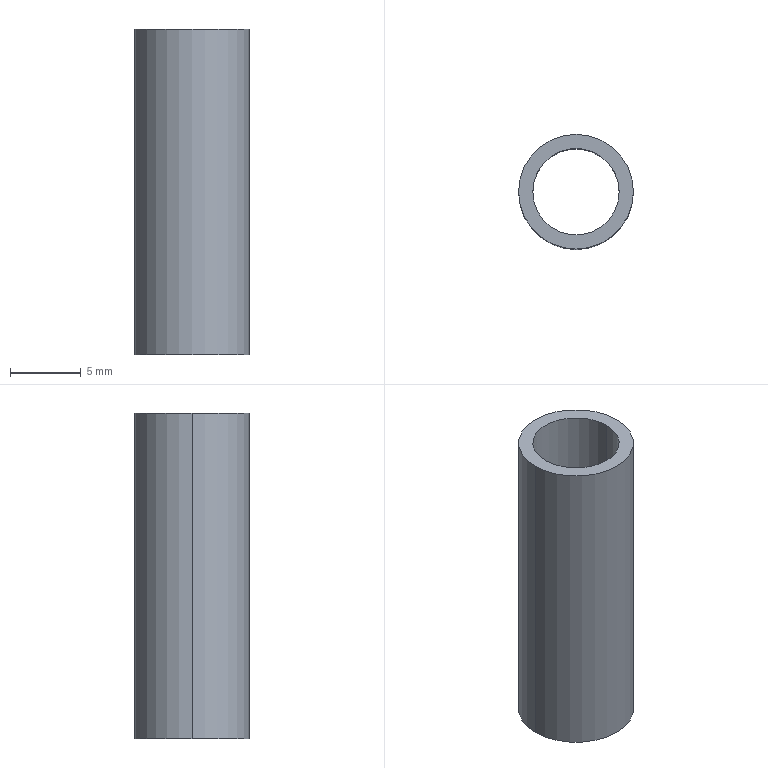Part | NX | features BREP 1 | 1 solid | 6 faces | box 8.1 x 8.1 x 23 mm | volume 513.022 mm3 | cylinder 4 | plane 2 | commonest cylinder face diameters 6.1 x2 8.1 x2
STEP:
#1=CARTESIAN_POINT('',(144.219,-518.178,23.));
#2=VERTEX_POINT('',#1);
#3=CARTESIAN_POINT('',(150.319,-518.178,23.));
#4=VERTEX_POINT('',#3);
#5=CARTESIAN_POINT('',(147.269,-518.178,23.));
#6=DIRECTION('',(0.,0.,1.));
#7=DIRECTION('',(0.,-1.,0.));
#8=AXIS2_PLACEMENT_3D('',#5,#6,#7);
#9=CIRCLE('',#8,3.05);
#10=EDGE_CURVE('',#2,#4,#9,.T.);
#11=ORIENTED_EDGE('',*,*,#10,.T.);
#12=CARTESIAN_POINT('',(150.319,-518.178,0.));
#13=VERTEX_POINT('',#12);
#14=CARTESIAN_POINT('',(150.319,-518.178,34.455));
#15=DIRECTION('',(0.,0.,-1.));
#16=VECTOR('',#15,1000.);
#17=LINE('',#14,#16);
#18=EDGE_CURVE('',#13,#4,#17,.F.);
#19=ORIENTED_EDGE('',*,*,#18,.F.);
#20=CARTESIAN_POINT('',(144.219,-518.178,0.));
#21=VERTEX_POINT('',#20);
#22=CARTESIAN_POINT('',(147.269,-518.178,0.));
#23=DIRECTION('',(0.,0.,1.));
#24=DIRECTION('',(1.,0.,0.));
#25=AXIS2_PLACEMENT_3D('',#22,#23,#24);
#26=CIRCLE('',#25,3.05);
#27=EDGE_CURVE('',#21,#13,#26,.T.);
#28=ORIENTED_EDGE('',*,*,#27,.F.);
#29=CARTESIAN_POINT('',(144.219,-518.178,34.455));
#30=DIRECTION('',(0.,0.,-1.));
#31=VECTOR('',#30,1000.);
#32=LINE('',#29,#31);
#33=EDGE_CURVE('',#21,#2,#32,.F.);
#34=ORIENTED_EDGE('',*,*,#33,.T.);
#35=EDGE_LOOP('',(#11,#19,#28,#34));
#36=FACE_BOUND('',#35,.T.);
#37=CARTESIAN_POINT('',(147.269,-518.178,34.455));
#38=DIRECTION('',(0.,0.,-1.));
#39=DIRECTION('',(1.,0.,0.));
#40=AXIS2_PLACEMENT_3D('',#37,#38,#39);
#41=CYLINDRICAL_SURFACE('',#40,3.05);
#42=ADVANCED_FACE('',(#36),#41,.F.);
#43=CARTESIAN_POINT('',(151.319,-518.178,23.));
#44=VERTEX_POINT('',#43);
#45=CARTESIAN_POINT('',(143.219,-518.178,23.));
#46=VERTEX_POINT('',#45);
#47=CARTESIAN_POINT('',(147.269,-518.178,23.));
#48=DIRECTION('',(0.,0.,1.));
#49=DIRECTION('',(0.,-1.,0.));
#50=AXIS2_PLACEMENT_3D('',#47,#48,#49);
#51=CIRCLE('',#50,4.05);
#52=EDGE_CURVE('',#44,#46,#51,.T.);
#53=ORIENTED_EDGE('',*,*,#52,.F.);
#54=CARTESIAN_POINT('',(151.319,-518.178,0.));
#55=VERTEX_POINT('',#54);
#56=CARTESIAN_POINT('',(151.319,-518.178,34.455));
#57=DIRECTION('',(0.,0.,-1.));
#58=VECTOR('',#57,1000.);
#59=LINE('',#56,#58);
#60=EDGE_CURVE('',#55,#44,#59,.F.);
#61=ORIENTED_EDGE('',*,*,#60,.F.);
#62=CARTESIAN_POINT('',(143.219,-518.178,0.));
#63=VERTEX_POINT('',#62);
#64=CARTESIAN_POINT('',(147.269,-518.178,0.));
#65=DIRECTION('',(0.,0.,1.));
#66=DIRECTION('',(1.,0.,0.));
#67=AXIS2_PLACEMENT_3D('',#64,#65,#66);
#68=CIRCLE('',#67,4.05);
#69=EDGE_CURVE('',#55,#63,#68,.T.);
#70=ORIENTED_EDGE('',*,*,#69,.T.);
#71=CARTESIAN_POINT('',(143.219,-518.178,34.455));
#72=DIRECTION('',(0.,0.,-1.));
#73=VECTOR('',#72,1000.);
#74=LINE('',#71,#73);
#75=EDGE_CURVE('',#63,#46,#74,.F.);
#76=ORIENTED_EDGE('',*,*,#75,.T.);
#77=EDGE_LOOP('',(#53,#61,#70,#76));
#78=FACE_BOUND('',#77,.T.);
#79=CARTESIAN_POINT('',(147.269,-518.178,34.455));
#80=DIRECTION('',(0.,0.,-1.));
#81=DIRECTION('',(1.,0.,0.));
#82=AXIS2_PLACEMENT_3D('',#79,#80,#81);
#83=CYLINDRICAL_SURFACE('',#82,4.05);
#84=ADVANCED_FACE('',(#78),#83,.T.);
#85=ORIENTED_EDGE('',*,*,#60,.T.);
#86=CARTESIAN_POINT('',(147.269,-518.178,23.));
#87=DIRECTION('',(0.,0.,1.));
#88=DIRECTION('',(0.,-1.,0.));
#89=AXIS2_PLACEMENT_3D('',#86,#87,#88);
#90=CIRCLE('',#89,4.05);
#91=EDGE_CURVE('',#46,#44,#90,.T.);
#92=ORIENTED_EDGE('',*,*,#91,.F.);
#93=ORIENTED_EDGE('',*,*,#75,.F.);
#94=CARTESIAN_POINT('',(147.269,-518.178,0.));
#95=DIRECTION('',(0.,0.,1.));
#96=DIRECTION('',(1.,0.,0.));
#97=AXIS2_PLACEMENT_3D('',#94,#95,#96);
#98=CIRCLE('',#97,4.05);
#99=EDGE_CURVE('',#63,#55,#98,.T.);
#100=ORIENTED_EDGE('',*,*,#99,.T.);
#101=EDGE_LOOP('',(#85,#92,#93,#100));
#102=FACE_BOUND('',#101,.T.);
#103=CARTESIAN_POINT('',(147.269,-518.178,34.455));
#104=DIRECTION('',(0.,0.,-1.));
#105=DIRECTION('',(1.,0.,0.));
#106=AXIS2_PLACEMENT_3D('',#103,#104,#105);
#107=CYLINDRICAL_SURFACE('',#106,4.05);
#108=ADVANCED_FACE('',(#102),#107,.T.);
#109=ORIENTED_EDGE('',*,*,#99,.F.);
#110=ORIENTED_EDGE('',*,*,#69,.F.);
#111=EDGE_LOOP('',(#109,#110));
#112=FACE_BOUND('',#111,.T.);
#113=ORIENTED_EDGE('',*,*,#27,.T.);
#114=CARTESIAN_POINT('',(147.269,-518.178,0.));
#115=DIRECTION('',(0.,0.,1.));
#116=DIRECTION('',(1.,0.,0.));
#117=AXIS2_PLACEMENT_3D('',#114,#115,#116);
#118=CIRCLE('',#117,3.05);
#119=EDGE_CURVE('',#13,#21,#118,.T.);
#120=ORIENTED_EDGE('',*,*,#119,.T.);
#121=EDGE_LOOP('',(#113,#120));
#122=FACE_BOUND('',#121,.T.);
#123=CARTESIAN_POINT('',(147.269,-518.178,0.));
#124=DIRECTION('',(0.,0.,1.));
#125=DIRECTION('',(-1.,0.,0.));
#126=AXIS2_PLACEMENT_3D('',#123,#124,#125);
#127=PLANE('',#126);
#128=ADVANCED_FACE('',(#112,#122),#127,.F.);
#129=ORIENTED_EDGE('',*,*,#18,.T.);
#130=CARTESIAN_POINT('',(147.269,-518.178,23.));
#131=DIRECTION('',(0.,0.,1.));
#132=DIRECTION('',(0.,-1.,0.));
#133=AXIS2_PLACEMENT_3D('',#130,#131,#132);
#134=CIRCLE('',#133,3.05);
#135=EDGE_CURVE('',#4,#2,#134,.T.);
#136=ORIENTED_EDGE('',*,*,#135,.T.);
#137=ORIENTED_EDGE('',*,*,#33,.F.);
#138=ORIENTED_EDGE('',*,*,#119,.F.);
#139=EDGE_LOOP('',(#129,#136,#137,#138));
#140=FACE_BOUND('',#139,.T.);
#141=CARTESIAN_POINT('',(147.269,-518.178,34.455));
#142=DIRECTION('',(0.,0.,-1.));
#143=DIRECTION('',(1.,0.,0.));
#144=AXIS2_PLACEMENT_3D('',#141,#142,#143);
#145=CYLINDRICAL_SURFACE('',#144,3.05);
#146=ADVANCED_FACE('',(#140),#145,.F.);
#147=ORIENTED_EDGE('',*,*,#91,.T.);
#148=ORIENTED_EDGE('',*,*,#52,.T.);
#149=EDGE_LOOP('',(#147,#148));
#150=FACE_BOUND('',#149,.T.);
#151=ORIENTED_EDGE('',*,*,#10,.F.);
#152=ORIENTED_EDGE('',*,*,#135,.F.);
#153=EDGE_LOOP('',(#151,#152));
#154=FACE_BOUND('',#153,.T.);
#155=CARTESIAN_POINT('',(142.543,-521.181,23.));
#156=DIRECTION('',(0.,0.,1.));
#157=DIRECTION('',(-1.,0.,0.));
#158=AXIS2_PLACEMENT_3D('',#155,#156,#157);
#159=PLANE('',#158);
#160=ADVANCED_FACE('',(#150,#154),#159,.T.);
#161=CLOSED_SHELL('',(#42,#84,#108,#128,#146,#160));
#162=MANIFOLD_SOLID_BREP('',#161);
#163=(LENGTH_UNIT()NAMED_UNIT(*)SI_UNIT(.MILLI.,.METRE.));
#164=UNCERTAINTY_MEASURE_WITH_UNIT(LENGTH_MEASURE(0.00001),#163,'','');
#165=(NAMED_UNIT(*)PLANE_ANGLE_UNIT()SI_UNIT($,.RADIAN.));
#166=(NAMED_UNIT(*)SI_UNIT($,.STERADIAN.)SOLID_ANGLE_UNIT());
#167=(GEOMETRIC_REPRESENTATION_CONTEXT(3)GLOBAL_UNCERTAINTY_ASSIGNED_CONTEXT((#164))GLOBAL_UNIT_ASSIGNED_CONTEXT((#163,#165,#166))REPRESENTATION_CONTEXT('',''));
#168=ADVANCED_BREP_SHAPE_REPRESENTATION('',(#162),#167);